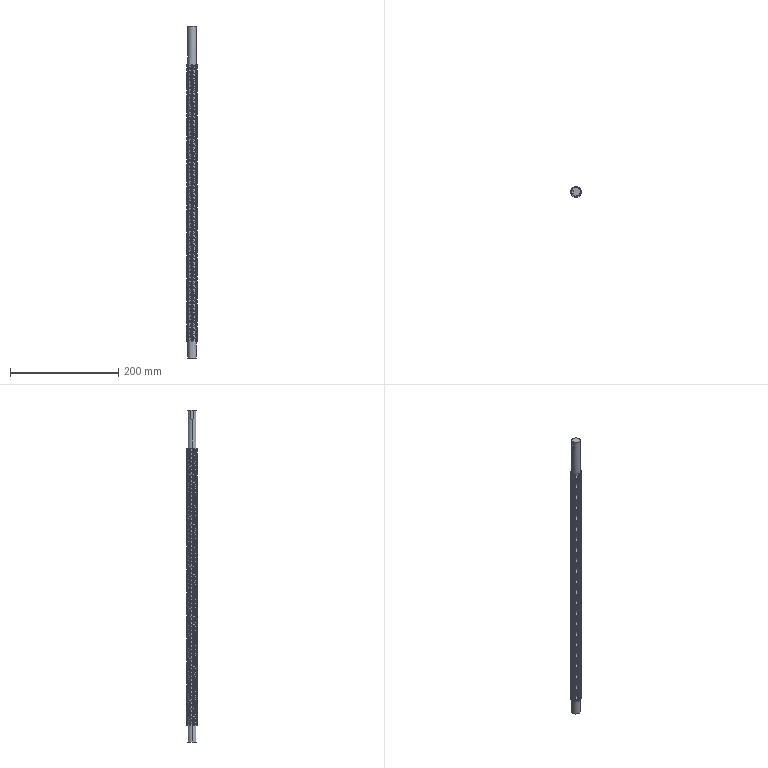Part | SolidWorks | features MoveFace 3, Cut 2, ICE 2, Extrusion 1, SweepThread 1 | 1 solid | 433 faces | box 20 x 20 x 613.565 mm | volume 157929 mm3 | cylinder 418 | plane 12 | spline 3 | commonest cylinder face diameters 20 x410 16 x4 4 x3 5 x1